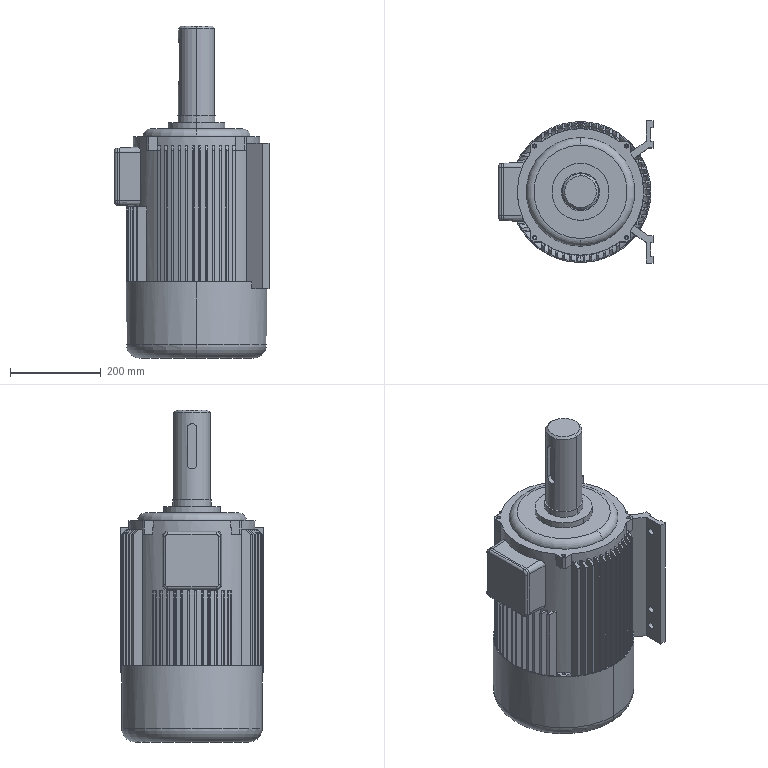Part | SolidWorks | 2 solids | 640 faces | box 340 x 314 x 732 mm | volume 11771559 mm3 | plane 308 | cylinder 175 | cone 145 | torus 12 | commonest cylinder face diameters 310 x50 6.8 x36 9 x16 10 x12 15 x12 279 x8